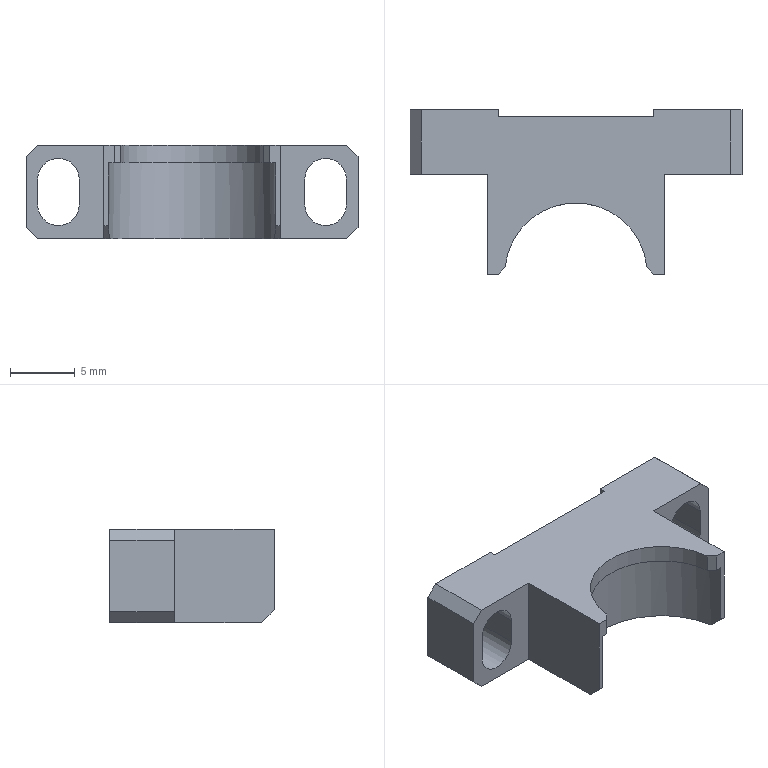Part | SolidWorks | features ICE 7, Chamfer 3, MoveFace 2, Extrusion 1 | 1 solid | 34 faces | box 25.6 x 12.7 x 7.2 mm | volume 1033 mm3 | plane 28 | cylinder 6 | commonest cylinder face diameters 3.2 x4 11 x1 12.9 x1
STEP:
#1=CARTESIAN_POINT('',(6.,12.7,6.85));
#2=VERTEX_POINT('',#1);
#3=CARTESIAN_POINT('',(6.,12.7,-0.35));
#4=VERTEX_POINT('',#3);
#5=CARTESIAN_POINT('',(6.,12.7,0.));
#6=DIRECTION('',(0.,0.,-1.));
#7=VECTOR('',#6,1000.);
#8=LINE('',#5,#7);
#9=EDGE_CURVE('',#2,#4,#8,.T.);
#10=ORIENTED_EDGE('',*,*,#9,.F.);
#11=CARTESIAN_POINT('',(11.945,12.7,6.85));
#12=VERTEX_POINT('',#11);
#13=CARTESIAN_POINT('',(0.,12.7,6.85));
#14=DIRECTION('',(-1.,0.,0.));
#15=VECTOR('',#14,1000.);
#16=LINE('',#13,#15);
#17=EDGE_CURVE('',#12,#2,#16,.T.);
#18=ORIENTED_EDGE('',*,*,#17,.F.);
#19=CARTESIAN_POINT('',(12.8,12.7,5.995));
#20=VERTEX_POINT('',#19);
#21=CARTESIAN_POINT('',(12.797,12.7,5.997));
#22=DIRECTION('',(0.7071,0.,-0.7071));
#23=VECTOR('',#22,1000.);
#24=LINE('',#21,#23);
#25=EDGE_CURVE('',#12,#20,#24,.T.);
#26=ORIENTED_EDGE('',*,*,#25,.T.);
#27=CARTESIAN_POINT('',(12.8,12.7,0.505));
#28=VERTEX_POINT('',#27);
#29=CARTESIAN_POINT('',(12.8,12.7,0.));
#30=DIRECTION('',(0.,0.,-1.));
#31=VECTOR('',#30,1000.);
#32=LINE('',#29,#31);
#33=EDGE_CURVE('',#20,#28,#32,.T.);
#34=ORIENTED_EDGE('',*,*,#33,.T.);
#35=CARTESIAN_POINT('',(11.945,12.7,-0.35));
#36=VERTEX_POINT('',#35);
#37=CARTESIAN_POINT('',(9.547,12.7,-2.747));
#38=DIRECTION('',(-0.7071,0.,-0.7071));
#39=VECTOR('',#38,1000.);
#40=LINE('',#37,#39);
#41=EDGE_CURVE('',#28,#36,#40,.T.);
#42=ORIENTED_EDGE('',*,*,#41,.T.);
#43=CARTESIAN_POINT('',(0.,12.7,-0.35));
#44=DIRECTION('',(-1.,0.,0.));
#45=VECTOR('',#44,1000.);
#46=LINE('',#43,#45);
#47=EDGE_CURVE('',#36,#4,#46,.T.);
#48=ORIENTED_EDGE('',*,*,#47,.T.);
#49=EDGE_LOOP('',(#10,#18,#26,#34,#42,#48));
#50=FACE_OUTER_BOUND('',#49,.T.);
#51=CARTESIAN_POINT('',(8.7,12.7,2.25));
#52=VERTEX_POINT('',#51);
#53=CARTESIAN_POINT('',(11.9,12.7,2.25));
#54=VERTEX_POINT('',#53);
#55=CARTESIAN_POINT('',(10.3,12.7,2.25));
#56=DIRECTION('',(0.,-1.,0.));
#57=DIRECTION('',(1.,0.,0.));
#58=AXIS2_PLACEMENT_3D('',#55,#56,#57);
#59=CIRCLE('',#58,1.6);
#60=EDGE_CURVE('',#52,#54,#59,.T.);
#61=ORIENTED_EDGE('',*,*,#60,.T.);
#62=CARTESIAN_POINT('',(11.9,12.7,4.25));
#63=VERTEX_POINT('',#62);
#64=CARTESIAN_POINT('',(11.9,12.7,2.25));
#65=DIRECTION('',(0.,0.,1.));
#66=VECTOR('',#65,1000.);
#67=LINE('',#64,#66);
#68=EDGE_CURVE('',#54,#63,#67,.T.);
#69=ORIENTED_EDGE('',*,*,#68,.T.);
#70=CARTESIAN_POINT('',(8.7,12.7,4.25));
#71=VERTEX_POINT('',#70);
#72=CARTESIAN_POINT('',(10.3,12.7,4.25));
#73=DIRECTION('',(0.,-1.,0.));
#74=DIRECTION('',(1.,0.,0.));
#75=AXIS2_PLACEMENT_3D('',#72,#73,#74);
#76=CIRCLE('',#75,1.6);
#77=EDGE_CURVE('',#63,#71,#76,.T.);
#78=ORIENTED_EDGE('',*,*,#77,.T.);
#79=CARTESIAN_POINT('',(8.7,12.7,2.25));
#80=DIRECTION('',(0.,0.,-1.));
#81=VECTOR('',#80,1000.);
#82=LINE('',#79,#81);
#83=EDGE_CURVE('',#71,#52,#82,.T.);
#84=ORIENTED_EDGE('',*,*,#83,.T.);
#85=EDGE_LOOP('',(#61,#69,#78,#84));
#86=FACE_BOUND('',#85,.T.);
#87=CARTESIAN_POINT('',(6.8,12.7,0.));
#88=DIRECTION('',(0.,1.,0.));
#89=DIRECTION('',(-1.,0.,0.));
#90=AXIS2_PLACEMENT_3D('',#87,#88,#89);
#91=PLANE('',#90);
#92=ADVANCED_FACE('',(#50,#86),#91,.T.);
#93=CARTESIAN_POINT('',(-6.8,7.7,-0.35));
#94=VERTEX_POINT('',#93);
#95=CARTESIAN_POINT('',(-6.8,1.,-0.35));
#96=VERTEX_POINT('',#95);
#97=CARTESIAN_POINT('',(-6.8,0.,-0.35));
#98=DIRECTION('',(0.,-1.,0.));
#99=VECTOR('',#98,1000.);
#100=LINE('',#97,#99);
#101=EDGE_CURVE('',#94,#96,#100,.T.);
#102=ORIENTED_EDGE('',*,*,#101,.T.);
#103=CARTESIAN_POINT('',(-6.8,0.,0.65));
#104=VERTEX_POINT('',#103);
#105=CARTESIAN_POINT('',(-6.8,0.325,0.325));
#106=DIRECTION('',(0.,-0.7071,0.7071));
#107=VECTOR('',#106,1000.);
#108=LINE('',#105,#107);
#109=EDGE_CURVE('',#96,#104,#108,.T.);
#110=ORIENTED_EDGE('',*,*,#109,.T.);
#111=CARTESIAN_POINT('',(-6.8,0.,6.85));
#112=VERTEX_POINT('',#111);
#113=CARTESIAN_POINT('',(-6.8,0.,0.));
#114=DIRECTION('',(0.,0.,1.));
#115=VECTOR('',#114,1000.);
#116=LINE('',#113,#115);
#117=EDGE_CURVE('',#104,#112,#116,.T.);
#118=ORIENTED_EDGE('',*,*,#117,.T.);
#119=CARTESIAN_POINT('',(-6.8,7.7,6.85));
#120=VERTEX_POINT('',#119);
#121=CARTESIAN_POINT('',(-6.8,0.,6.85));
#122=DIRECTION('',(0.,-1.,0.));
#123=VECTOR('',#122,1000.);
#124=LINE('',#121,#123);
#125=EDGE_CURVE('',#120,#112,#124,.T.);
#126=ORIENTED_EDGE('',*,*,#125,.F.);
#127=CARTESIAN_POINT('',(-6.8,7.7,6.5));
#128=DIRECTION('',(0.,0.,-1.));
#129=VECTOR('',#128,1000.);
#130=LINE('',#127,#129);
#131=EDGE_CURVE('',#120,#94,#130,.T.);
#132=ORIENTED_EDGE('',*,*,#131,.T.);
#133=EDGE_LOOP('',(#102,#110,#118,#126,#132));
#134=FACE_OUTER_BOUND('',#133,.T.);
#135=CARTESIAN_POINT('',(-6.8,0.,0.));
#136=DIRECTION('',(-1.,0.,0.));
#137=DIRECTION('',(0.,0.,1.));
#138=AXIS2_PLACEMENT_3D('',#135,#136,#137);
#139=PLANE('',#138);
#140=ADVANCED_FACE('',(#134),#139,.T.);
#141=CARTESIAN_POINT('',(6.8,0.,0.65));
#142=VERTEX_POINT('',#141);
#143=CARTESIAN_POINT('',(6.8,0.,6.85));
#144=VERTEX_POINT('',#143);
#145=CARTESIAN_POINT('',(6.8,0.,0.));
#146=DIRECTION('',(0.,0.,1.));
#147=VECTOR('',#146,1000.);
#148=LINE('',#145,#147);
#149=EDGE_CURVE('',#142,#144,#148,.T.);
#150=ORIENTED_EDGE('',*,*,#149,.F.);
#151=CARTESIAN_POINT('',(6.8,1.,-0.35));
#152=VERTEX_POINT('',#151);
#153=CARTESIAN_POINT('',(6.8,0.325,0.325));
#154=DIRECTION('',(0.,0.7071,-0.7071));
#155=VECTOR('',#154,1000.);
#156=LINE('',#153,#155);
#157=EDGE_CURVE('',#142,#152,#156,.T.);
#158=ORIENTED_EDGE('',*,*,#157,.T.);
#159=CARTESIAN_POINT('',(6.8,7.7,-0.35));
#160=VERTEX_POINT('',#159);
#161=CARTESIAN_POINT('',(6.8,0.,-0.35));
#162=DIRECTION('',(0.,1.,0.));
#163=VECTOR('',#162,1000.);
#164=LINE('',#161,#163);
#165=EDGE_CURVE('',#152,#160,#164,.T.);
#166=ORIENTED_EDGE('',*,*,#165,.T.);
#167=CARTESIAN_POINT('',(6.8,7.7,6.85));
#168=VERTEX_POINT('',#167);
#169=CARTESIAN_POINT('',(6.8,7.7,0.));
#170=DIRECTION('',(0.,0.,1.));
#171=VECTOR('',#170,1000.);
#172=LINE('',#169,#171);
#173=EDGE_CURVE('',#160,#168,#172,.T.);
#174=ORIENTED_EDGE('',*,*,#173,.T.);
#175=CARTESIAN_POINT('',(6.8,0.,6.85));
#176=DIRECTION('',(0.,1.,0.));
#177=VECTOR('',#176,1000.);
#178=LINE('',#175,#177);
#179=EDGE_CURVE('',#144,#168,#178,.T.);
#180=ORIENTED_EDGE('',*,*,#179,.F.);
#181=EDGE_LOOP('',(#150,#158,#166,#174,#180));
#182=FACE_OUTER_BOUND('',#181,.T.);
#183=CARTESIAN_POINT('',(6.8,0.,0.));
#184=DIRECTION('',(1.,0.,0.));
#185=DIRECTION('',(0.,0.,-1.));
#186=AXIS2_PLACEMENT_3D('',#183,#184,#185);
#187=PLANE('',#186);
#188=ADVANCED_FACE('',(#182),#187,.T.);
#189=CARTESIAN_POINT('',(5.475,0.5251,5.5));
#190=VERTEX_POINT('',#189);
#191=CARTESIAN_POINT('',(-5.475,0.5251,5.5));
#192=VERTEX_POINT('',#191);
#193=CARTESIAN_POINT('',(0.,0.,5.5));
#194=DIRECTION('',(0.,0.,1.));
#195=DIRECTION('',(-1.,0.,0.));
#196=AXIS2_PLACEMENT_3D('',#193,#194,#195);
#197=CIRCLE('',#196,5.5);
#198=EDGE_CURVE('',#190,#192,#197,.T.);
#199=ORIENTED_EDGE('',*,*,#198,.F.);
#200=CARTESIAN_POINT('',(5.475,0.5251,6.85));
#201=VERTEX_POINT('',#200);
#202=CARTESIAN_POINT('',(5.475,0.5251,10.));
#203=DIRECTION('',(0.,0.,1.));
#204=VECTOR('',#203,1000.);
#205=LINE('',#202,#204);
#206=EDGE_CURVE('',#190,#201,#205,.T.);
#207=ORIENTED_EDGE('',*,*,#206,.T.);
#208=CARTESIAN_POINT('',(-5.475,0.5251,6.85));
#209=VERTEX_POINT('',#208);
#210=CARTESIAN_POINT('',(0.,0.,6.85));
#211=DIRECTION('',(0.,0.,1.));
#212=DIRECTION('',(1.,0.,0.));
#213=AXIS2_PLACEMENT_3D('',#210,#211,#212);
#214=CIRCLE('',#213,5.5);
#215=EDGE_CURVE('',#201,#209,#214,.T.);
#216=ORIENTED_EDGE('',*,*,#215,.T.);
#217=CARTESIAN_POINT('',(-5.475,0.5251,10.));
#218=DIRECTION('',(0.,0.,-1.));
#219=VECTOR('',#218,1000.);
#220=LINE('',#217,#219);
#221=EDGE_CURVE('',#209,#192,#220,.T.);
#222=ORIENTED_EDGE('',*,*,#221,.T.);
#223=EDGE_LOOP('',(#199,#207,#216,#222));
#224=FACE_OUTER_BOUND('',#223,.T.);
#225=CARTESIAN_POINT('',(0.,0.,10.));
#226=DIRECTION('',(0.,0.,-1.));
#227=DIRECTION('',(-1.,0.,0.));
#228=AXIS2_PLACEMENT_3D('',#225,#226,#227);
#229=CYLINDRICAL_SURFACE('',#228,5.5);
#230=ADVANCED_FACE('',(#224),#229,.F.);
#231=ORIENTED_EDGE('',*,*,#215,.F.);
#232=CARTESIAN_POINT('',(6.,0.,6.85));
#233=VERTEX_POINT('',#232);
#234=CARTESIAN_POINT('',(3.,3.,6.85));
#235=DIRECTION('',(0.7071,-0.7071,0.));
#236=VECTOR('',#235,1000.);
#237=LINE('',#234,#236);
#238=EDGE_CURVE('',#201,#233,#237,.T.);
#239=ORIENTED_EDGE('',*,*,#238,.T.);
#240=CARTESIAN_POINT('',(0.,0.,6.85));
#241=DIRECTION('',(-1.,0.,0.));
#242=VECTOR('',#241,1000.);
#243=LINE('',#240,#242);
#244=EDGE_CURVE('',#144,#233,#243,.T.);
#245=ORIENTED_EDGE('',*,*,#244,.F.);
#246=ORIENTED_EDGE('',*,*,#179,.T.);
#247=CARTESIAN_POINT('',(11.945,7.7,6.85));
#248=VERTEX_POINT('',#247);
#249=CARTESIAN_POINT('',(0.,7.7,6.85));
#250=DIRECTION('',(1.,0.,0.));
#251=VECTOR('',#250,1000.);
#252=LINE('',#249,#251);
#253=EDGE_CURVE('',#168,#248,#252,.T.);
#254=ORIENTED_EDGE('',*,*,#253,.T.);
#255=CARTESIAN_POINT('',(11.945,0.,6.85));
#256=DIRECTION('',(0.,1.,0.));
#257=VECTOR('',#256,1000.);
#258=LINE('',#255,#257);
#259=EDGE_CURVE('',#248,#12,#258,.T.);
#260=ORIENTED_EDGE('',*,*,#259,.T.);
#261=ORIENTED_EDGE('',*,*,#17,.T.);
#262=CARTESIAN_POINT('',(6.,12.2,6.85));
#263=VERTEX_POINT('',#262);
#264=CARTESIAN_POINT('',(6.,0.,6.85));
#265=DIRECTION('',(0.,1.,0.));
#266=VECTOR('',#265,1000.);
#267=LINE('',#264,#266);
#268=EDGE_CURVE('',#263,#2,#267,.T.);
#269=ORIENTED_EDGE('',*,*,#268,.F.);
#270=CARTESIAN_POINT('',(-6.,12.2,6.85));
#271=VERTEX_POINT('',#270);
#272=CARTESIAN_POINT('',(0.,12.2,6.85));
#273=DIRECTION('',(1.,0.,0.));
#274=VECTOR('',#273,1000.);
#275=LINE('',#272,#274);
#276=EDGE_CURVE('',#271,#263,#275,.T.);
#277=ORIENTED_EDGE('',*,*,#276,.F.);
#278=CARTESIAN_POINT('',(-6.,12.7,6.85));
#279=VERTEX_POINT('',#278);
#280=CARTESIAN_POINT('',(-6.,12.2,6.85));
#281=DIRECTION('',(0.,1.,0.));
#282=VECTOR('',#281,1000.);
#283=LINE('',#280,#282);
#284=EDGE_CURVE('',#271,#279,#283,.T.);
#285=ORIENTED_EDGE('',*,*,#284,.T.);
#286=CARTESIAN_POINT('',(-11.945,12.7,6.85));
#287=VERTEX_POINT('',#286);
#288=CARTESIAN_POINT('',(0.,12.7,6.85));
#289=DIRECTION('',(-1.,0.,0.));
#290=VECTOR('',#289,1000.);
#291=LINE('',#288,#290);
#292=EDGE_CURVE('',#279,#287,#291,.T.);
#293=ORIENTED_EDGE('',*,*,#292,.T.);
#294=CARTESIAN_POINT('',(-11.945,7.7,6.85));
#295=VERTEX_POINT('',#294);
#296=CARTESIAN_POINT('',(-11.945,0.,6.85));
#297=DIRECTION('',(0.,-1.,0.));
#298=VECTOR('',#297,1000.);
#299=LINE('',#296,#298);
#300=EDGE_CURVE('',#287,#295,#299,.T.);
#301=ORIENTED_EDGE('',*,*,#300,.T.);
#302=CARTESIAN_POINT('',(0.,7.7,6.85));
#303=DIRECTION('',(1.,0.,0.));
#304=VECTOR('',#303,1000.);
#305=LINE('',#302,#304);
#306=EDGE_CURVE('',#295,#120,#305,.T.);
#307=ORIENTED_EDGE('',*,*,#306,.T.);
#308=ORIENTED_EDGE('',*,*,#125,.T.);
#309=CARTESIAN_POINT('',(-6.,0.,6.85));
#310=VERTEX_POINT('',#309);
#311=CARTESIAN_POINT('',(0.,0.,6.85));
#312=DIRECTION('',(-1.,0.,0.));
#313=VECTOR('',#312,1000.);
#314=LINE('',#311,#313);
#315=EDGE_CURVE('',#310,#112,#314,.T.);
#316=ORIENTED_EDGE('',*,*,#315,.F.);
#317=CARTESIAN_POINT('',(-3.,3.,6.85));
#318=DIRECTION('',(0.7071,0.7071,0.));
#319=VECTOR('',#318,1000.);
#320=LINE('',#317,#319);
#321=EDGE_CURVE('',#310,#209,#320,.T.);
#322=ORIENTED_EDGE('',*,*,#321,.T.);
#323=EDGE_LOOP('',(#231,#239,#245,#246,#254,#260,#261,#269,#277,#285,#293,#301,#307,#308,#316,#322));
#324=FACE_OUTER_BOUND('',#323,.T.);
#325=CARTESIAN_POINT('',(0.,0.,6.85));
#326=DIRECTION('',(0.,0.,1.));
#327=DIRECTION('',(1.,0.,0.));
#328=AXIS2_PLACEMENT_3D('',#325,#326,#327);
#329=PLANE('',#328);
#330=ADVANCED_FACE('',(#324),#329,.T.);
#331=ORIENTED_EDGE('',*,*,#165,.F.);
#332=CARTESIAN_POINT('',(6.372,1.,-0.35));
#333=VERTEX_POINT('',#332);
#334=CARTESIAN_POINT('',(0.,1.,-0.35));
#335=DIRECTION('',(-1.,0.,0.));
#336=VECTOR('',#335,1000.);
#337=LINE('',#334,#336);
#338=EDGE_CURVE('',#152,#333,#337,.T.);
#339=ORIENTED_EDGE('',*,*,#338,.T.);
#340=CARTESIAN_POINT('',(-6.372,1.,-0.35));
#341=VERTEX_POINT('',#340);
#342=CARTESIAN_POINT('',(0.,0.,-0.35));
#343=DIRECTION('',(0.,0.,-1.));
#344=DIRECTION('',(1.,0.,0.));
#345=AXIS2_PLACEMENT_3D('',#342,#343,#344);
#346=CIRCLE('',#345,6.45);
#347=EDGE_CURVE('',#341,#333,#346,.T.);
#348=ORIENTED_EDGE('',*,*,#347,.F.);
#349=CARTESIAN_POINT('',(0.,1.,-0.35));
#350=DIRECTION('',(-1.,0.,0.));
#351=VECTOR('',#350,1000.);
#352=LINE('',#349,#351);
#353=EDGE_CURVE('',#341,#96,#352,.T.);
#354=ORIENTED_EDGE('',*,*,#353,.T.);
#355=ORIENTED_EDGE('',*,*,#101,.F.);
#356=CARTESIAN_POINT('',(-11.945,7.7,-0.35));
#357=VERTEX_POINT('',#356);
#358=CARTESIAN_POINT('',(0.,7.7,-0.35));
#359=DIRECTION('',(-1.,0.,0.));
#360=VECTOR('',#359,1000.);
#361=LINE('',#358,#360);
#362=EDGE_CURVE('',#94,#357,#361,.T.);
#363=ORIENTED_EDGE('',*,*,#362,.T.);
#364=CARTESIAN_POINT('',(-11.945,12.7,-0.35));
#365=VERTEX_POINT('',#364);
#366=CARTESIAN_POINT('',(-11.945,0.,-0.35));
#367=DIRECTION('',(0.,1.,0.));
#368=VECTOR('',#367,1000.);
#369=LINE('',#366,#368);
#370=EDGE_CURVE('',#357,#365,#369,.T.);
#371=ORIENTED_EDGE('',*,*,#370,.T.);
#372=CARTESIAN_POINT('',(-6.,12.7,-0.35));
#373=VERTEX_POINT('',#372);
#374=CARTESIAN_POINT('',(0.,12.7,-0.35));
#375=DIRECTION('',(-1.,0.,0.));
#376=VECTOR('',#375,1000.);
#377=LINE('',#374,#376);
#378=EDGE_CURVE('',#373,#365,#377,.T.);
#379=ORIENTED_EDGE('',*,*,#378,.F.);
#380=CARTESIAN_POINT('',(-6.,12.2,-0.35));
#381=VERTEX_POINT('',#380);
#382=CARTESIAN_POINT('',(-6.,12.2,-0.35));
#383=DIRECTION('',(0.,1.,0.));
#384=VECTOR('',#383,1000.);
#385=LINE('',#382,#384);
#386=EDGE_CURVE('',#381,#373,#385,.T.);
#387=ORIENTED_EDGE('',*,*,#386,.F.);
#388=CARTESIAN_POINT('',(6.,12.2,-0.35));
#389=VERTEX_POINT('',#388);
#390=CARTESIAN_POINT('',(0.,12.2,-0.35));
#391=DIRECTION('',(-1.,0.,0.));
#392=VECTOR('',#391,1000.);
#393=LINE('',#390,#392);
#394=EDGE_CURVE('',#389,#381,#393,.T.);
#395=ORIENTED_EDGE('',*,*,#394,.F.);
#396=CARTESIAN_POINT('',(6.,0.,-0.35));
#397=DIRECTION('',(0.,1.,0.));
#398=VECTOR('',#397,1000.);
#399=LINE('',#396,#398);
#400=EDGE_CURVE('',#389,#4,#399,.T.);
#401=ORIENTED_EDGE('',*,*,#400,.T.);
#402=ORIENTED_EDGE('',*,*,#47,.F.);
#403=CARTESIAN_POINT('',(11.945,7.7,-0.35));
#404=VERTEX_POINT('',#403);
#405=CARTESIAN_POINT('',(11.945,7.7,-0.35));
#406=DIRECTION('',(0.,-1.,0.));
#407=VECTOR('',#406,1000.);
#408=LINE('',#405,#407);
#409=EDGE_CURVE('',#36,#404,#408,.T.);
#410=ORIENTED_EDGE('',*,*,#409,.T.);
#411=CARTESIAN_POINT('',(0.,7.7,-0.35));
#412=DIRECTION('',(-1.,0.,0.));
#413=VECTOR('',#412,1000.);
#414=LINE('',#411,#413);
#415=EDGE_CURVE('',#404,#160,#414,.T.);
#416=ORIENTED_EDGE('',*,*,#415,.T.);
#417=EDGE_LOOP('',(#331,#339,#348,#354,#355,#363,#371,#379,#387,#395,#401,#402,#410,#416));
#418=FACE_OUTER_BOUND('',#417,.T.);
#419=CARTESIAN_POINT('',(0.,0.,-0.35));
#420=DIRECTION('',(0.,0.,1.));
#421=DIRECTION('',(1.,0.,0.));
#422=AXIS2_PLACEMENT_3D('',#419,#420,#421);
#423=PLANE('',#422);
#424=ADVANCED_FACE('',(#418),#423,.F.);
#425=CARTESIAN_POINT('',(6.,0.,5.5));
#426=VERTEX_POINT('',#425);
#427=CARTESIAN_POINT('',(6.45,0.,5.5));
#428=VERTEX_POINT('',#427);
#429=CARTESIAN_POINT('',(0.,0.,5.5));
#430=DIRECTION('',(1.,0.,0.));
#431=VECTOR('',#430,1000.);
#432=LINE('',#429,#431);
#433=EDGE_CURVE('',#426,#428,#432,.T.);
#434=ORIENTED_EDGE('',*,*,#433,.F.);
#435=CARTESIAN_POINT('',(3.,3.,5.5));
#436=DIRECTION('',(-0.7071,0.7071,0.));
#437=VECTOR('',#436,1000.);
#438=LINE('',#435,#437);
#439=EDGE_CURVE('',#426,#190,#438,.T.);
#440=ORIENTED_EDGE('',*,*,#439,.T.);
#441=ORIENTED_EDGE('',*,*,#198,.T.);
#442=CARTESIAN_POINT('',(-6.,0.,5.5));
#443=VERTEX_POINT('',#442);
#444=CARTESIAN_POINT('',(-3.,3.,5.5));
#445=DIRECTION('',(-0.7071,-0.7071,0.));
#446=VECTOR('',#445,1000.);
#447=LINE('',#444,#446);
#448=EDGE_CURVE('',#192,#443,#447,.T.);
#449=ORIENTED_EDGE('',*,*,#448,.T.);
#450=CARTESIAN_POINT('',(-6.45,0.,5.5));
#451=VERTEX_POINT('',#450);
#452=CARTESIAN_POINT('',(0.,0.,5.5));
#453=DIRECTION('',(1.,0.,0.));
#454=VECTOR('',#453,1000.);
#455=LINE('',#452,#454);
#456=EDGE_CURVE('',#451,#443,#455,.T.);
#457=ORIENTED_EDGE('',*,*,#456,.F.);
#458=CARTESIAN_POINT('',(0.,0.,5.5));
#459=DIRECTION('',(0.,0.,-1.));
#460=DIRECTION('',(-1.,0.,0.));
#461=AXIS2_PLACEMENT_3D('',#458,#459,#460);
#462=CIRCLE('',#461,6.45);
#463=EDGE_CURVE('',#451,#428,#462,.T.);
#464=ORIENTED_EDGE('',*,*,#463,.T.);
#465=EDGE_LOOP('',(#434,#440,#441,#449,#457,#464));
#466=FACE_OUTER_BOUND('',#465,.T.);
#467=CARTESIAN_POINT('',(0.,0.,5.5));
#468=DIRECTION('',(0.,0.,-1.));
#469=DIRECTION('',(-1.,0.,0.));
#470=AXIS2_PLACEMENT_3D('',#467,#468,#469);
#471=PLANE('',#470);
#472=ADVANCED_FACE('',(#466),#471,.T.);
#473=ORIENTED_EDGE('',*,*,#347,.T.);
#474=CARTESIAN_POINT('',(6.45,0.,0.65));
#475=VERTEX_POINT('',#474);
#476=CARTESIAN_POINT('',(6.372,1.,-0.35));
#477=CARTESIAN_POINT('',(6.424,0.669,-0.01903));
#478=CARTESIAN_POINT('',(6.45,0.335,0.315));
#479=CARTESIAN_POINT('',(6.45,0.,0.65));
#480=(BOUNDED_CURVE()B_SPLINE_CURVE(3,(#476,#477,#478,#479),.UNSPECIFIED.,.F.,.F.)B_SPLINE_CURVE_WITH_KNOTS((4,4),(1.415,1.571),.UNSPECIFIED.)CURVE()GEOMETRIC_REPRESENTATION_ITEM()RATIONAL_B_SPLINE_CURVE((1.,0.998,0.998,1.))REPRESENTATION_ITEM(''));
#481=EDGE_CURVE('',#333,#475,#480,.T.);
#482=ORIENTED_EDGE('',*,*,#481,.T.);
#483=CARTESIAN_POINT('',(6.45,0.,5.5));
#484=DIRECTION('',(0.,0.,1.));
#485=VECTOR('',#484,1000.);
#486=LINE('',#483,#485);
#487=EDGE_CURVE('',#475,#428,#486,.T.);
#488=ORIENTED_EDGE('',*,*,#487,.T.);
#489=ORIENTED_EDGE('',*,*,#463,.F.);
#490=CARTESIAN_POINT('',(-6.45,0.,0.65));
#491=VERTEX_POINT('',#490);
#492=CARTESIAN_POINT('',(-6.45,0.,5.5));
#493=DIRECTION('',(0.,0.,-1.));
#494=VECTOR('',#493,1000.);
#495=LINE('',#492,#494);
#496=EDGE_CURVE('',#451,#491,#495,.T.);
#497=ORIENTED_EDGE('',*,*,#496,.T.);
#498=CARTESIAN_POINT('',(-6.45,0.,0.65));
#499=CARTESIAN_POINT('',(-6.45,0.335,0.315));
#500=CARTESIAN_POINT('',(-6.424,0.669,-0.01903));
#501=CARTESIAN_POINT('',(-6.372,1.,-0.35));
#502=(BOUNDED_CURVE()B_SPLINE_CURVE(3,(#498,#499,#500,#501),.UNSPECIFIED.,.F.,.F.)B_SPLINE_CURVE_WITH_KNOTS((4,4),(4.712,4.868),.UNSPECIFIED.)CURVE()GEOMETRIC_REPRESENTATION_ITEM()RATIONAL_B_SPLINE_CURVE((1.,0.998,0.998,1.))REPRESENTATION_ITEM(''));
#503=EDGE_CURVE('',#491,#341,#502,.T.);
#504=ORIENTED_EDGE('',*,*,#503,.T.);
#505=EDGE_LOOP('',(#473,#482,#488,#489,#497,#504));
#506=FACE_OUTER_BOUND('',#505,.T.);
#507=CARTESIAN_POINT('',(0.,0.,5.5));
#508=DIRECTION('',(0.,0.,-1.));
#509=DIRECTION('',(-1.,0.,0.));
#510=AXIS2_PLACEMENT_3D('',#507,#508,#509);
#511=CYLINDRICAL_SURFACE('',#510,6.45);
#512=ADVANCED_FACE('',(#506),#511,.F.);
#513=CARTESIAN_POINT('',(-6.,12.7,6.5));
#514=DIRECTION('',(0.,0.,1.));
#515=VECTOR('',#514,1000.);
#516=LINE('',#513,#515);
#517=EDGE_CURVE('',#373,#279,#516,.T.);
#518=ORIENTED_EDGE('',*,*,#517,.F.);
#519=ORIENTED_EDGE('',*,*,#378,.T.);
#520=CARTESIAN_POINT('',(-12.8,12.7,0.505));
#521=VERTEX_POINT('',#520);
#522=CARTESIAN_POINT('',(-2.747,12.7,-9.547));
#523=DIRECTION('',(-0.7071,0.,0.7071));
#524=VECTOR('',#523,1000.);
#525=LINE('',#522,#524);
#526=EDGE_CURVE('',#365,#521,#525,.T.);
#527=ORIENTED_EDGE('',*,*,#526,.T.);
#528=CARTESIAN_POINT('',(-12.8,12.7,5.995));
#529=VERTEX_POINT('',#528);
#530=CARTESIAN_POINT('',(-12.8,12.7,6.5));
#531=DIRECTION('',(0.,0.,1.));
#532=VECTOR('',#531,1000.);
#533=LINE('',#530,#532);
#534=EDGE_CURVE('',#521,#529,#533,.T.);
#535=ORIENTED_EDGE('',*,*,#534,.T.);
#536=CARTESIAN_POINT('',(-5.997,12.7,12.797));
#537=DIRECTION('',(0.7071,0.,0.7071));
#538=VECTOR('',#537,1000.);
#539=LINE('',#536,#538);
#540=EDGE_CURVE('',#529,#287,#539,.T.);
#541=ORIENTED_EDGE('',*,*,#540,.T.);
#542=ORIENTED_EDGE('',*,*,#292,.F.);
#543=EDGE_LOOP('',(#518,#519,#527,#535,#541,#542));
#544=FACE_OUTER_BOUND('',#543,.T.);
#545=CARTESIAN_POINT('',(-8.7,12.7,4.25));
#546=VERTEX_POINT('',#545);
#547=CARTESIAN_POINT('',(-11.9,12.7,4.25));
#548=VERTEX_POINT('',#547);
#549=CARTESIAN_POINT('',(-10.3,12.7,4.25));
#550=DIRECTION('',(0.,-1.,0.));
#551=DIRECTION('',(-1.,0.,0.));
#552=AXIS2_PLACEMENT_3D('',#549,#550,#551);
#553=CIRCLE('',#552,1.6);
#554=EDGE_CURVE('',#546,#548,#553,.T.);
#555=ORIENTED_EDGE('',*,*,#554,.T.);
#556=CARTESIAN_POINT('',(-11.9,12.7,2.25));
#557=VERTEX_POINT('',#556);
#558=CARTESIAN_POINT('',(-11.9,12.7,2.25));
#559=DIRECTION('',(0.,0.,-1.));
#560=VECTOR('',#559,1000.);
#561=LINE('',#558,#560);
#562=EDGE_CURVE('',#548,#557,#561,.T.);
#563=ORIENTED_EDGE('',*,*,#562,.T.);
#564=CARTESIAN_POINT('',(-8.7,12.7,2.25));
#565=VERTEX_POINT('',#564);
#566=CARTESIAN_POINT('',(-10.3,12.7,2.25));
#567=DIRECTION('',(0.,-1.,0.));
#568=DIRECTION('',(-1.,0.,0.));
#569=AXIS2_PLACEMENT_3D('',#566,#567,#568);
#570=CIRCLE('',#569,1.6);
#571=EDGE_CURVE('',#557,#565,#570,.T.);
#572=ORIENTED_EDGE('',*,*,#571,.T.);
#573=CARTESIAN_POINT('',(-8.7,12.7,2.25));
#574=DIRECTION('',(0.,0.,1.));
#575=VECTOR('',#574,1000.);
#576=LINE('',#573,#575);
#577=EDGE_CURVE('',#565,#546,#576,.T.);
#578=ORIENTED_EDGE('',*,*,#577,.T.);
#579=EDGE_LOOP('',(#555,#563,#572,#578));
#580=FACE_BOUND('',#579,.T.);
#581=CARTESIAN_POINT('',(6.8,12.7,0.));
#582=DIRECTION('',(0.,1.,0.));
#583=DIRECTION('',(-1.,0.,0.));
#584=AXIS2_PLACEMENT_3D('',#581,#582,#583);
#585=PLANE('',#584);
#586=ADVANCED_FACE('',(#544,#580),#585,.T.);
#587=CARTESIAN_POINT('',(12.8,7.7,5.995));
#588=VERTEX_POINT('',#587);
#589=CARTESIAN_POINT('',(12.8,7.7,0.505));
#590=VERTEX_POINT('',#589);
#591=CARTESIAN_POINT('',(12.8,7.7,0.));
#592=DIRECTION('',(0.,0.,-1.));
#593=VECTOR('',#592,1000.);
#594=LINE('',#591,#593);
#595=EDGE_CURVE('',#588,#590,#594,.T.);
#596=ORIENTED_EDGE('',*,*,#595,.T.);
#597=CARTESIAN_POINT('',(12.8,7.7,0.505));
#598=DIRECTION('',(0.,1.,0.));
#599=VECTOR('',#598,1000.);
#600=LINE('',#597,#599);
#601=EDGE_CURVE('',#590,#28,#600,.T.);
#602=ORIENTED_EDGE('',*,*,#601,.T.);
#603=ORIENTED_EDGE('',*,*,#33,.F.);
#604=CARTESIAN_POINT('',(12.8,7.7,5.995));
#605=DIRECTION('',(0.,-1.,0.));
#606=VECTOR('',#605,1000.);
#607=LINE('',#604,#606);
#608=EDGE_CURVE('',#20,#588,#607,.T.);
#609=ORIENTED_EDGE('',*,*,#608,.T.);
#610=EDGE_LOOP('',(#596,#602,#603,#609));
#611=FACE_OUTER_BOUND('',#610,.T.);
#612=CARTESIAN_POINT('',(12.8,7.7,0.));
#613=DIRECTION('',(1.,0.,0.));
#614=DIRECTION('',(0.,0.,-1.));
#615=AXIS2_PLACEMENT_3D('',#612,#613,#614);
#616=PLANE('',#615);
#617=ADVANCED_FACE('',(#611),#616,.T.);
#618=CARTESIAN_POINT('',(11.9,7.7,2.25));
#619=VERTEX_POINT('',#618);
#620=CARTESIAN_POINT('',(11.9,7.7,4.25));
#621=VERTEX_POINT('',#620);
#622=CARTESIAN_POINT('',(11.9,7.7,2.25));
#623=DIRECTION('',(0.,0.,1.));
#624=VECTOR('',#623,1000.);
#625=LINE('',#622,#624);
#626=EDGE_CURVE('',#619,#621,#625,.T.);
#627=ORIENTED_EDGE('',*,*,#626,.F.);
#628=CARTESIAN_POINT('',(8.7,7.7,2.25));
#629=VERTEX_POINT('',#628);
#630=CARTESIAN_POINT('',(10.3,7.7,2.25));
#631=DIRECTION('',(0.,-1.,0.));
#632=DIRECTION('',(1.,0.,0.));
#633=AXIS2_PLACEMENT_3D('',#630,#631,#632);
#634=CIRCLE('',#633,1.6);
#635=EDGE_CURVE('',#629,#619,#634,.T.);
#636=ORIENTED_EDGE('',*,*,#635,.F.);
#637=CARTESIAN_POINT('',(8.7,7.7,4.25));
#638=VERTEX_POINT('',#637);
#639=CARTESIAN_POINT('',(8.7,7.7,2.25));
#640=DIRECTION('',(0.,0.,-1.));
#641=VECTOR('',#640,1000.);
#642=LINE('',#639,#641);
#643=EDGE_CURVE('',#638,#629,#642,.T.);
#644=ORIENTED_EDGE('',*,*,#643,.F.);
#645=CARTESIAN_POINT('',(10.3,7.7,4.25));
#646=DIRECTION('',(0.,-1.,0.));
#647=DIRECTION('',(1.,0.,0.));
#648=AXIS2_PLACEMENT_3D('',#645,#646,#647);
#649=CIRCLE('',#648,1.6);
#650=EDGE_CURVE('',#621,#638,#649,.T.);
#651=ORIENTED_EDGE('',*,*,#650,.F.);
#652=EDGE_LOOP('',(#627,#636,#644,#651));
#653=FACE_BOUND('',#652,.T.);
#654=ORIENTED_EDGE('',*,*,#415,.F.);
#655=CARTESIAN_POINT('',(13.047,7.7,0.7525));
#656=DIRECTION('',(0.7071,0.,0.7071));
#657=VECTOR('',#656,1000.);
#658=LINE('',#655,#657);
#659=EDGE_CURVE('',#404,#590,#658,.T.);
#660=ORIENTED_EDGE('',*,*,#659,.T.);
#661=ORIENTED_EDGE('',*,*,#595,.F.);
#662=CARTESIAN_POINT('',(12.047,7.7,6.747));
#663=DIRECTION('',(-0.7071,0.,0.7071));
#664=VECTOR('',#663,1000.);
#665=LINE('',#662,#664);
#666=EDGE_CURVE('',#588,#248,#665,.T.);
#667=ORIENTED_EDGE('',*,*,#666,.T.);
#668=ORIENTED_EDGE('',*,*,#253,.F.);
#669=ORIENTED_EDGE('',*,*,#173,.F.);
#670=EDGE_LOOP('',(#654,#660,#661,#667,#668,#669));
#671=FACE_OUTER_BOUND('',#670,.T.);
#672=CARTESIAN_POINT('',(0.,7.7,0.));
#673=DIRECTION('',(0.,1.,0.));
#674=DIRECTION('',(-1.,0.,0.));
#675=AXIS2_PLACEMENT_3D('',#672,#673,#674);
#676=PLANE('',#675);
#677=ADVANCED_FACE('',(#653,#671),#676,.F.);
#678=CARTESIAN_POINT('',(-12.8,7.7,0.505));
#679=VERTEX_POINT('',#678);
#680=CARTESIAN_POINT('',(-12.8,7.7,5.995));
#681=VERTEX_POINT('',#680);
#682=CARTESIAN_POINT('',(-12.8,7.7,6.5));
#683=DIRECTION('',(0.,0.,1.));
#684=VECTOR('',#683,1000.);
#685=LINE('',#682,#684);
#686=EDGE_CURVE('',#679,#681,#685,.T.);
#687=ORIENTED_EDGE('',*,*,#686,.T.);
#688=CARTESIAN_POINT('',(-12.8,7.7,5.995));
#689=DIRECTION('',(0.,1.,0.));
#690=VECTOR('',#689,1000.);
#691=LINE('',#688,#690);
#692=EDGE_CURVE('',#681,#529,#691,.T.);
#693=ORIENTED_EDGE('',*,*,#692,.T.);
#694=ORIENTED_EDGE('',*,*,#534,.F.);
#695=CARTESIAN_POINT('',(-12.8,7.7,0.505));
#696=DIRECTION('',(0.,-1.,0.));
#697=VECTOR('',#696,1000.);
#698=LINE('',#695,#697);
#699=EDGE_CURVE('',#521,#679,#698,.T.);
#700=ORIENTED_EDGE('',*,*,#699,.T.);
#701=EDGE_LOOP('',(#687,#693,#694,#700));
#702=FACE_OUTER_BOUND('',#701,.T.);
#703=CARTESIAN_POINT('',(-12.8,7.7,6.5));
#704=DIRECTION('',(-1.,0.,0.));
#705=DIRECTION('',(0.,-1.,0.));
#706=AXIS2_PLACEMENT_3D('',#703,#704,#705);
#707=PLANE('',#706);
#708=ADVANCED_FACE('',(#702),#707,.T.);
#709=CARTESIAN_POINT('',(-11.9,7.7,4.25));
#710=VERTEX_POINT('',#709);
#711=CARTESIAN_POINT('',(-11.9,7.7,2.25));
#712=VERTEX_POINT('',#711);
#713=CARTESIAN_POINT('',(-11.9,7.7,2.25));
#714=DIRECTION('',(0.,0.,-1.));
#715=VECTOR('',#714,1000.);
#716=LINE('',#713,#715);
#717=EDGE_CURVE('',#710,#712,#716,.T.);
#718=ORIENTED_EDGE('',*,*,#717,.F.);
#719=CARTESIAN_POINT('',(-8.7,7.7,4.25));
#720=VERTEX_POINT('',#719);
#721=CARTESIAN_POINT('',(-10.3,7.7,4.25));
#722=DIRECTION('',(0.,-1.,0.));
#723=DIRECTION('',(-1.,0.,0.));
#724=AXIS2_PLACEMENT_3D('',#721,#722,#723);
#725=CIRCLE('',#724,1.6);
#726=EDGE_CURVE('',#720,#710,#725,.T.);
#727=ORIENTED_EDGE('',*,*,#726,.F.);
#728=CARTESIAN_POINT('',(-8.7,7.7,2.25));
#729=VERTEX_POINT('',#728);
#730=CARTESIAN_POINT('',(-8.7,7.7,2.25));
#731=DIRECTION('',(0.,0.,1.));
#732=VECTOR('',#731,1000.);
#733=LINE('',#730,#732);
#734=EDGE_CURVE('',#729,#720,#733,.T.);
#735=ORIENTED_EDGE('',*,*,#734,.F.);
#736=CARTESIAN_POINT('',(-10.3,7.7,2.25));
#737=DIRECTION('',(0.,-1.,0.));
#738=DIRECTION('',(-1.,0.,0.));
#739=AXIS2_PLACEMENT_3D('',#736,#737,#738);
#740=CIRCLE('',#739,1.6);
#741=EDGE_CURVE('',#712,#729,#740,.T.);
#742=ORIENTED_EDGE('',*,*,#741,.F.);
#743=EDGE_LOOP('',(#718,#727,#735,#742));
#744=FACE_BOUND('',#743,.T.);
#745=ORIENTED_EDGE('',*,*,#306,.F.);
#746=CARTESIAN_POINT('',(-13.047,7.7,5.747));
#747=DIRECTION('',(-0.7071,0.,-0.7071));
#748=VECTOR('',#747,1000.);
#749=LINE('',#746,#748);
#750=EDGE_CURVE('',#295,#681,#749,.T.);
#751=ORIENTED_EDGE('',*,*,#750,.T.);
#752=ORIENTED_EDGE('',*,*,#686,.F.);
#753=CARTESIAN_POINT('',(-12.047,7.7,-0.2475));
#754=DIRECTION('',(0.7071,0.,-0.7071));
#755=VECTOR('',#754,1000.);
#756=LINE('',#753,#755);
#757=EDGE_CURVE('',#679,#357,#756,.T.);
#758=ORIENTED_EDGE('',*,*,#757,.T.);
#759=ORIENTED_EDGE('',*,*,#362,.F.);
#760=ORIENTED_EDGE('',*,*,#131,.F.);
#761=EDGE_LOOP('',(#745,#751,#752,#758,#759,#760));
#762=FACE_OUTER_BOUND('',#761,.T.);
#763=CARTESIAN_POINT('',(0.,7.7,0.));
#764=DIRECTION('',(0.,1.,0.));
#765=DIRECTION('',(-1.,0.,0.));
#766=AXIS2_PLACEMENT_3D('',#763,#764,#765);
#767=PLANE('',#766);
#768=ADVANCED_FACE('',(#744,#762),#767,.F.);
#769=ORIENTED_EDGE('',*,*,#726,.T.);
#770=CARTESIAN_POINT('',(-11.9,12.7,4.25));
#771=DIRECTION('',(0.,-1.,0.));
#772=VECTOR('',#771,1000.);
#773=LINE('',#770,#772);
#774=EDGE_CURVE('',#548,#710,#773,.T.);
#775=ORIENTED_EDGE('',*,*,#774,.F.);
#776=ORIENTED_EDGE('',*,*,#554,.F.);
#777=CARTESIAN_POINT('',(-8.7,12.7,4.25));
#778=DIRECTION('',(0.,-1.,0.));
#779=VECTOR('',#778,1000.);
#780=LINE('',#777,#779);
#781=EDGE_CURVE('',#546,#720,#780,.T.);
#782=ORIENTED_EDGE('',*,*,#781,.T.);
#783=EDGE_LOOP('',(#769,#775,#776,#782));
#784=FACE_OUTER_BOUND('',#783,.T.);
#785=CARTESIAN_POINT('',(-10.3,12.7,4.25));
#786=DIRECTION('',(0.,-1.,0.));
#787=DIRECTION('',(1.,0.,0.));
#788=AXIS2_PLACEMENT_3D('',#785,#786,#787);
#789=CYLINDRICAL_SURFACE('',#788,1.6);
#790=ADVANCED_FACE('',(#784),#789,.F.);
#791=ORIENTED_EDGE('',*,*,#734,.T.);
#792=ORIENTED_EDGE('',*,*,#781,.F.);
#793=ORIENTED_EDGE('',*,*,#577,.F.);
#794=CARTESIAN_POINT('',(-8.7,12.7,2.25));
#795=DIRECTION('',(0.,-1.,0.));
#796=VECTOR('',#795,1000.);
#797=LINE('',#794,#796);
#798=EDGE_CURVE('',#565,#729,#797,.T.);
#799=ORIENTED_EDGE('',*,*,#798,.T.);
#800=EDGE_LOOP('',(#791,#792,#793,#799));
#801=FACE_OUTER_BOUND('',#800,.T.);
#802=CARTESIAN_POINT('',(-8.7,12.7,2.25));
#803=DIRECTION('',(1.,0.,0.));
#804=DIRECTION('',(0.,1.,0.));
#805=AXIS2_PLACEMENT_3D('',#802,#803,#804);
#806=PLANE('',#805);
#807=ADVANCED_FACE('',(#801),#806,.F.);
#808=ORIENTED_EDGE('',*,*,#741,.T.);
#809=ORIENTED_EDGE('',*,*,#798,.F.);
#810=ORIENTED_EDGE('',*,*,#571,.F.);
#811=CARTESIAN_POINT('',(-11.9,12.7,2.25));
#812=DIRECTION('',(0.,-1.,0.));
#813=VECTOR('',#812,1000.);
#814=LINE('',#811,#813);
#815=EDGE_CURVE('',#557,#712,#814,.T.);
#816=ORIENTED_EDGE('',*,*,#815,.T.);
#817=EDGE_LOOP('',(#808,#809,#810,#816));
#818=FACE_OUTER_BOUND('',#817,.T.);
#819=CARTESIAN_POINT('',(-10.3,12.7,2.25));
#820=DIRECTION('',(0.,-1.,0.));
#821=DIRECTION('',(1.,0.,0.));
#822=AXIS2_PLACEMENT_3D('',#819,#820,#821);
#823=CYLINDRICAL_SURFACE('',#822,1.6);
#824=ADVANCED_FACE('',(#818),#823,.F.);
#825=ORIENTED_EDGE('',*,*,#717,.T.);
#826=ORIENTED_EDGE('',*,*,#815,.F.);
#827=ORIENTED_EDGE('',*,*,#562,.F.);
#828=ORIENTED_EDGE('',*,*,#774,.T.);
#829=EDGE_LOOP('',(#825,#826,#827,#828));
#830=FACE_OUTER_BOUND('',#829,.T.);
#831=CARTESIAN_POINT('',(-11.9,12.7,2.25));
#832=DIRECTION('',(-1.,0.,0.));
#833=DIRECTION('',(0.,-1.,0.));
#834=AXIS2_PLACEMENT_3D('',#831,#832,#833);
#835=PLANE('',#834);
#836=ADVANCED_FACE('',(#830),#835,.F.);
#837=ORIENTED_EDGE('',*,*,#635,.T.);
#838=CARTESIAN_POINT('',(11.9,12.7,2.25));
#839=DIRECTION('',(0.,-1.,0.));
#840=VECTOR('',#839,1000.);
#841=LINE('',#838,#840);
#842=EDGE_CURVE('',#54,#619,#841,.T.);
#843=ORIENTED_EDGE('',*,*,#842,.F.);
#844=ORIENTED_EDGE('',*,*,#60,.F.);
#845=CARTESIAN_POINT('',(8.7,12.7,2.25));
#846=DIRECTION('',(0.,-1.,0.));
#847=VECTOR('',#846,1000.);
#848=LINE('',#845,#847);
#849=EDGE_CURVE('',#52,#629,#848,.T.);
#850=ORIENTED_EDGE('',*,*,#849,.T.);
#851=EDGE_LOOP('',(#837,#843,#844,#850));
#852=FACE_OUTER_BOUND('',#851,.T.);
#853=CARTESIAN_POINT('',(10.3,12.7,2.25));
#854=DIRECTION('',(0.,-1.,0.));
#855=DIRECTION('',(1.,0.,0.));
#856=AXIS2_PLACEMENT_3D('',#853,#854,#855);
#857=CYLINDRICAL_SURFACE('',#856,1.6);
#858=ADVANCED_FACE('',(#852),#857,.F.);
#859=ORIENTED_EDGE('',*,*,#643,.T.);
#860=ORIENTED_EDGE('',*,*,#849,.F.);
#861=ORIENTED_EDGE('',*,*,#83,.F.);
#862=CARTESIAN_POINT('',(8.7,12.7,4.25));
#863=DIRECTION('',(0.,-1.,0.));
#864=VECTOR('',#863,1000.);
#865=LINE('',#862,#864);
#866=EDGE_CURVE('',#71,#638,#865,.T.);
#867=ORIENTED_EDGE('',*,*,#866,.T.);
#868=EDGE_LOOP('',(#859,#860,#861,#867));
#869=FACE_OUTER_BOUND('',#868,.T.);
#870=CARTESIAN_POINT('',(8.7,12.7,2.25));
#871=DIRECTION('',(-1.,0.,0.));
#872=DIRECTION('',(0.,-1.,0.));
#873=AXIS2_PLACEMENT_3D('',#870,#871,#872);
#874=PLANE('',#873);
#875=ADVANCED_FACE('',(#869),#874,.F.);
#876=ORIENTED_EDGE('',*,*,#650,.T.);
#877=ORIENTED_EDGE('',*,*,#866,.F.);
#878=ORIENTED_EDGE('',*,*,#77,.F.);
#879=CARTESIAN_POINT('',(11.9,12.7,4.25));
#880=DIRECTION('',(0.,-1.,0.));
#881=VECTOR('',#880,1000.);
#882=LINE('',#879,#881);
#883=EDGE_CURVE('',#63,#621,#882,.T.);
#884=ORIENTED_EDGE('',*,*,#883,.T.);
#885=EDGE_LOOP('',(#876,#877,#878,#884));
#886=FACE_OUTER_BOUND('',#885,.T.);
#887=CARTESIAN_POINT('',(10.3,12.7,4.25));
#888=DIRECTION('',(0.,-1.,0.));
#889=DIRECTION('',(1.,0.,0.));
#890=AXIS2_PLACEMENT_3D('',#887,#888,#889);
#891=CYLINDRICAL_SURFACE('',#890,1.6);
#892=ADVANCED_FACE('',(#886),#891,.F.);
#893=ORIENTED_EDGE('',*,*,#626,.T.);
#894=ORIENTED_EDGE('',*,*,#883,.F.);
#895=ORIENTED_EDGE('',*,*,#68,.F.);
#896=ORIENTED_EDGE('',*,*,#842,.T.);
#897=EDGE_LOOP('',(#893,#894,#895,#896));
#898=FACE_OUTER_BOUND('',#897,.T.);
#899=CARTESIAN_POINT('',(11.9,12.7,2.25));
#900=DIRECTION('',(1.,0.,0.));
#901=DIRECTION('',(0.,1.,0.));
#902=AXIS2_PLACEMENT_3D('',#899,#900,#901);
#903=PLANE('',#902);
#904=ADVANCED_FACE('',(#898),#903,.F.);
#905=ORIENTED_EDGE('',*,*,#456,.T.);
#906=CARTESIAN_POINT('',(-6.,0.,10.));
#907=DIRECTION('',(0.,0.,1.));
#908=VECTOR('',#907,1000.);
#909=LINE('',#906,#908);
#910=EDGE_CURVE('',#443,#310,#909,.T.);
#911=ORIENTED_EDGE('',*,*,#910,.T.);
#912=ORIENTED_EDGE('',*,*,#315,.T.);
#913=ORIENTED_EDGE('',*,*,#117,.F.);
#914=CARTESIAN_POINT('',(-6.8,0.,0.65));
#915=DIRECTION('',(1.,0.,0.));
#916=VECTOR('',#915,1000.);
#917=LINE('',#914,#916);
#918=EDGE_CURVE('',#104,#491,#917,.T.);
#919=ORIENTED_EDGE('',*,*,#918,.T.);
#920=ORIENTED_EDGE('',*,*,#496,.F.);
#921=EDGE_LOOP('',(#905,#911,#912,#913,#919,#920));
#922=FACE_OUTER_BOUND('',#921,.T.);
#923=CARTESIAN_POINT('',(-6.8,0.,10.));
#924=DIRECTION('',(0.,1.,0.));
#925=DIRECTION('',(-1.,0.,0.));
#926=AXIS2_PLACEMENT_3D('',#923,#924,#925);
#927=PLANE('',#926);
#928=ADVANCED_FACE('',(#922),#927,.F.);
#929=ORIENTED_EDGE('',*,*,#244,.T.);
#930=CARTESIAN_POINT('',(6.,0.,10.));
#931=DIRECTION('',(0.,0.,-1.));
#932=VECTOR('',#931,1000.);
#933=LINE('',#930,#932);
#934=EDGE_CURVE('',#233,#426,#933,.T.);
#935=ORIENTED_EDGE('',*,*,#934,.T.);
#936=ORIENTED_EDGE('',*,*,#433,.T.);
#937=ORIENTED_EDGE('',*,*,#487,.F.);
#938=CARTESIAN_POINT('',(-6.8,0.,0.65));
#939=DIRECTION('',(1.,0.,0.));
#940=VECTOR('',#939,1000.);
#941=LINE('',#938,#940);
#942=EDGE_CURVE('',#475,#142,#941,.T.);
#943=ORIENTED_EDGE('',*,*,#942,.T.);
#944=ORIENTED_EDGE('',*,*,#149,.T.);
#945=EDGE_LOOP('',(#929,#935,#936,#937,#943,#944));
#946=FACE_OUTER_BOUND('',#945,.T.);
#947=CARTESIAN_POINT('',(-6.8,0.,10.));
#948=DIRECTION('',(0.,1.,0.));
#949=DIRECTION('',(-1.,0.,0.));
#950=AXIS2_PLACEMENT_3D('',#947,#948,#949);
#951=PLANE('',#950);
#952=ADVANCED_FACE('',(#946),#951,.F.);
#953=ORIENTED_EDGE('',*,*,#659,.F.);
#954=ORIENTED_EDGE('',*,*,#409,.F.);
#955=ORIENTED_EDGE('',*,*,#41,.F.);
#956=ORIENTED_EDGE('',*,*,#601,.F.);
#957=EDGE_LOOP('',(#953,#954,#955,#956));
#958=FACE_OUTER_BOUND('',#957,.T.);
#959=CARTESIAN_POINT('',(13.047,7.7,0.7525));
#960=DIRECTION('',(0.7071,0.,-0.7071));
#961=DIRECTION('',(0.,-1.,0.));
#962=AXIS2_PLACEMENT_3D('',#959,#960,#961);
#963=PLANE('',#962);
#964=ADVANCED_FACE('',(#958),#963,.T.);
#965=ORIENTED_EDGE('',*,*,#666,.F.);
#966=ORIENTED_EDGE('',*,*,#608,.F.);
#967=ORIENTED_EDGE('',*,*,#25,.F.);
#968=ORIENTED_EDGE('',*,*,#259,.F.);
#969=EDGE_LOOP('',(#965,#966,#967,#968));
#970=FACE_OUTER_BOUND('',#969,.T.);
#971=CARTESIAN_POINT('',(12.047,0.,6.747));
#972=DIRECTION('',(-0.7071,0.,-0.7071));
#973=DIRECTION('',(0.,1.,0.));
#974=AXIS2_PLACEMENT_3D('',#971,#972,#973);
#975=PLANE('',#974);
#976=ADVANCED_FACE('',(#970),#975,.F.);
#977=ORIENTED_EDGE('',*,*,#750,.F.);
#978=ORIENTED_EDGE('',*,*,#300,.F.);
#979=ORIENTED_EDGE('',*,*,#540,.F.);
#980=ORIENTED_EDGE('',*,*,#692,.F.);
#981=EDGE_LOOP('',(#977,#978,#979,#980));
#982=FACE_OUTER_BOUND('',#981,.T.);
#983=CARTESIAN_POINT('',(-13.047,7.7,5.747));
#984=DIRECTION('',(0.7071,0.,-0.7071));
#985=DIRECTION('',(0.,1.,0.));
#986=AXIS2_PLACEMENT_3D('',#983,#984,#985);
#987=PLANE('',#986);
#988=ADVANCED_FACE('',(#982),#987,.F.);
#989=ORIENTED_EDGE('',*,*,#757,.F.);
#990=ORIENTED_EDGE('',*,*,#699,.F.);
#991=ORIENTED_EDGE('',*,*,#526,.F.);
#992=ORIENTED_EDGE('',*,*,#370,.F.);
#993=EDGE_LOOP('',(#989,#990,#991,#992));
#994=FACE_OUTER_BOUND('',#993,.T.);
#995=CARTESIAN_POINT('',(-12.047,0.,-0.2475));
#996=DIRECTION('',(-0.7071,0.,-0.7071));
#997=DIRECTION('',(0.,-1.,0.));
#998=AXIS2_PLACEMENT_3D('',#995,#996,#997);
#999=PLANE('',#998);
#1000=ADVANCED_FACE('',(#994),#999,.T.);
#1001=ORIENTED_EDGE('',*,*,#9,.T.);
#1002=ORIENTED_EDGE('',*,*,#400,.F.);
#1003=CARTESIAN_POINT('',(6.,12.2,0.));
#1004=DIRECTION('',(0.,0.,-1.));
#1005=VECTOR('',#1004,1000.);
#1006=LINE('',#1003,#1005);
#1007=EDGE_CURVE('',#263,#389,#1006,.T.);
#1008=ORIENTED_EDGE('',*,*,#1007,.F.);
#1009=ORIENTED_EDGE('',*,*,#268,.T.);
#1010=EDGE_LOOP('',(#1001,#1002,#1008,#1009));
#1011=FACE_OUTER_BOUND('',#1010,.T.);
#1012=CARTESIAN_POINT('',(6.,12.2,0.));
#1013=DIRECTION('',(1.,0.,0.));
#1014=DIRECTION('',(0.,1.,0.));
#1015=AXIS2_PLACEMENT_3D('',#1012,#1013,#1014);
#1016=PLANE('',#1015);
#1017=ADVANCED_FACE('',(#1011),#1016,.F.);
#1018=ORIENTED_EDGE('',*,*,#517,.T.);
#1019=ORIENTED_EDGE('',*,*,#284,.F.);
#1020=CARTESIAN_POINT('',(-6.,12.2,6.5));
#1021=DIRECTION('',(0.,0.,1.));
#1022=VECTOR('',#1021,1000.);
#1023=LINE('',#1020,#1022);
#1024=EDGE_CURVE('',#381,#271,#1023,.T.);
#1025=ORIENTED_EDGE('',*,*,#1024,.F.);
#1026=ORIENTED_EDGE('',*,*,#386,.T.);
#1027=EDGE_LOOP('',(#1018,#1019,#1025,#1026));
#1028=FACE_OUTER_BOUND('',#1027,.T.);
#1029=CARTESIAN_POINT('',(-6.,12.2,6.5));
#1030=DIRECTION('',(-1.,0.,0.));
#1031=DIRECTION('',(0.,-1.,0.));
#1032=AXIS2_PLACEMENT_3D('',#1029,#1030,#1031);
#1033=PLANE('',#1032);
#1034=ADVANCED_FACE('',(#1028),#1033,.F.);
#1035=ORIENTED_EDGE('',*,*,#394,.T.);
#1036=ORIENTED_EDGE('',*,*,#1024,.T.);
#1037=ORIENTED_EDGE('',*,*,#276,.T.);
#1038=ORIENTED_EDGE('',*,*,#1007,.T.);
#1039=EDGE_LOOP('',(#1035,#1036,#1037,#1038));
#1040=FACE_OUTER_BOUND('',#1039,.T.);
#1041=CARTESIAN_POINT('',(0.,12.2,0.));
#1042=DIRECTION('',(0.,-1.,0.));
#1043=DIRECTION('',(1.,0.,0.));
#1044=AXIS2_PLACEMENT_3D('',#1041,#1042,#1043);
#1045=PLANE('',#1044);
#1046=ADVANCED_FACE('',(#1040),#1045,.F.);
#1047=ORIENTED_EDGE('',*,*,#481,.F.);
#1048=ORIENTED_EDGE('',*,*,#338,.F.);
#1049=ORIENTED_EDGE('',*,*,#157,.F.);
#1050=ORIENTED_EDGE('',*,*,#942,.F.);
#1051=EDGE_LOOP('',(#1047,#1048,#1049,#1050));
#1052=FACE_OUTER_BOUND('',#1051,.T.);
#1053=CARTESIAN_POINT('',(-6.8,0.,0.65));
#1054=DIRECTION('',(0.,0.7071,0.7071));
#1055=DIRECTION('',(1.,0.,0.));
#1056=AXIS2_PLACEMENT_3D('',#1053,#1054,#1055);
#1057=PLANE('',#1056);
#1058=ADVANCED_FACE('',(#1052),#1057,.F.);
#1059=ORIENTED_EDGE('',*,*,#109,.F.);
#1060=ORIENTED_EDGE('',*,*,#353,.F.);
#1061=ORIENTED_EDGE('',*,*,#503,.F.);
#1062=ORIENTED_EDGE('',*,*,#918,.F.);
#1063=EDGE_LOOP('',(#1059,#1060,#1061,#1062));
#1064=FACE_OUTER_BOUND('',#1063,.T.);
#1065=CARTESIAN_POINT('',(-6.8,0.,0.65));
#1066=DIRECTION('',(0.,0.7071,0.7071));
#1067=DIRECTION('',(1.,0.,0.));
#1068=AXIS2_PLACEMENT_3D('',#1065,#1066,#1067);
#1069=PLANE('',#1068);
#1070=ADVANCED_FACE('',(#1064),#1069,.F.);
#1071=ORIENTED_EDGE('',*,*,#439,.F.);
#1072=ORIENTED_EDGE('',*,*,#934,.F.);
#1073=ORIENTED_EDGE('',*,*,#238,.F.);
#1074=ORIENTED_EDGE('',*,*,#206,.F.);
#1075=EDGE_LOOP('',(#1071,#1072,#1073,#1074));
#1076=FACE_OUTER_BOUND('',#1075,.T.);
#1077=CARTESIAN_POINT('',(5.475,0.5251,10.));
#1078=DIRECTION('',(-0.7071,-0.7071,0.));
#1079=DIRECTION('',(0.,0.,-1.));
#1080=AXIS2_PLACEMENT_3D('',#1077,#1078,#1079);
#1081=PLANE('',#1080);
#1082=ADVANCED_FACE('',(#1076),#1081,.T.);
#1083=ORIENTED_EDGE('',*,*,#321,.F.);
#1084=ORIENTED_EDGE('',*,*,#910,.F.);
#1085=ORIENTED_EDGE('',*,*,#448,.F.);
#1086=ORIENTED_EDGE('',*,*,#221,.F.);
#1087=EDGE_LOOP('',(#1083,#1084,#1085,#1086));
#1088=FACE_OUTER_BOUND('',#1087,.T.);
#1089=CARTESIAN_POINT('',(-5.475,0.5251,10.));
#1090=DIRECTION('',(-0.7071,0.7071,0.));
#1091=DIRECTION('',(0.,0.,-1.));
#1092=AXIS2_PLACEMENT_3D('',#1089,#1090,#1091);
#1093=PLANE('',#1092);
#1094=ADVANCED_FACE('',(#1088),#1093,.F.);
#1095=CLOSED_SHELL('',(#92,#140,#188,#230,#330,#424,#472,#512,#586,#617,#677,#708,#768,#790,#807,#824,#836,#858,#875,#892,#904,#928,#952,#964,#976,#988,#1000,#1017,#1034,#1046,#1058,#1070,#1082,#1094));
#1096=MANIFOLD_SOLID_BREP('',#1095);
#1097=CARTESIAN_POINT('',(0.,0.,0.));
#1098=DIRECTION('',(0.,0.,1.));
#1099=DIRECTION('',(1.,0.,0.));
#1100=AXIS2_PLACEMENT_3D('',#1097,#1098,#1099);
#1101=(LENGTH_UNIT()NAMED_UNIT(*)SI_UNIT(.MILLI.,.METRE.));
#1102=UNCERTAINTY_MEASURE_WITH_UNIT(LENGTH_MEASURE(0.00001),#1101,'','');
#1103=(NAMED_UNIT(*)PLANE_ANGLE_UNIT()SI_UNIT($,.RADIAN.));
#1104=(NAMED_UNIT(*)SI_UNIT($,.STERADIAN.)SOLID_ANGLE_UNIT());
#1105=(GEOMETRIC_REPRESENTATION_CONTEXT(3)GLOBAL_UNCERTAINTY_ASSIGNED_CONTEXT((#1102))GLOBAL_UNIT_ASSIGNED_CONTEXT((#1101,#1103,#1104))REPRESENTATION_CONTEXT('',''));
#1106=ADVANCED_BREP_SHAPE_REPRESENTATION('',(#1096,#1100),#1105);